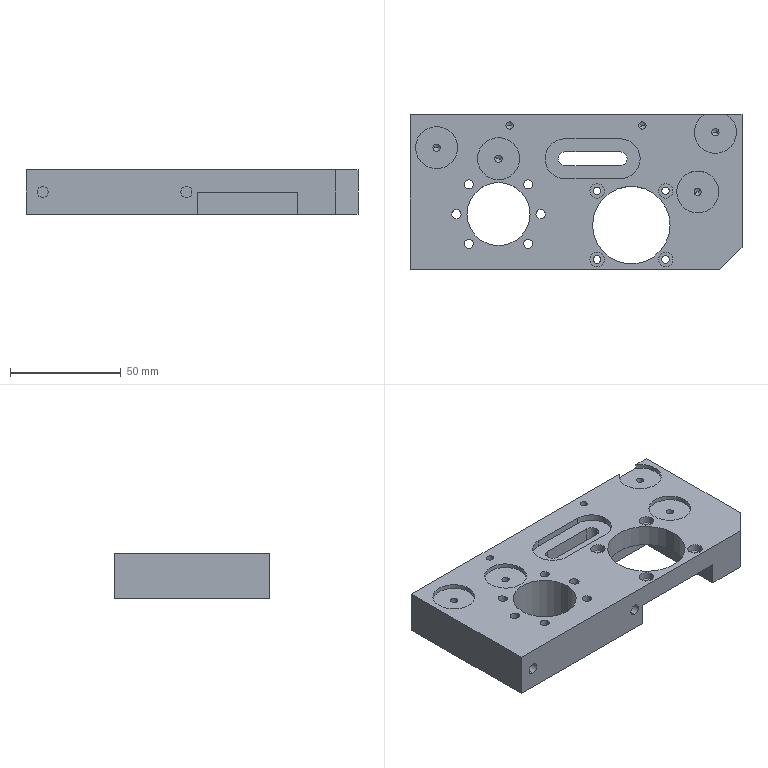Part | STEP file | Rear rail (right) | 1 solid | 119 faces | box 150 x 70 x 20 mm | volume 154483 mm3 | cylinder 72 | plane 29 | cone 18 | commonest cylinder face diameters 4.2 x18 3.3 x12 19 x9 3.4 x8 6.5 x8 5 x4